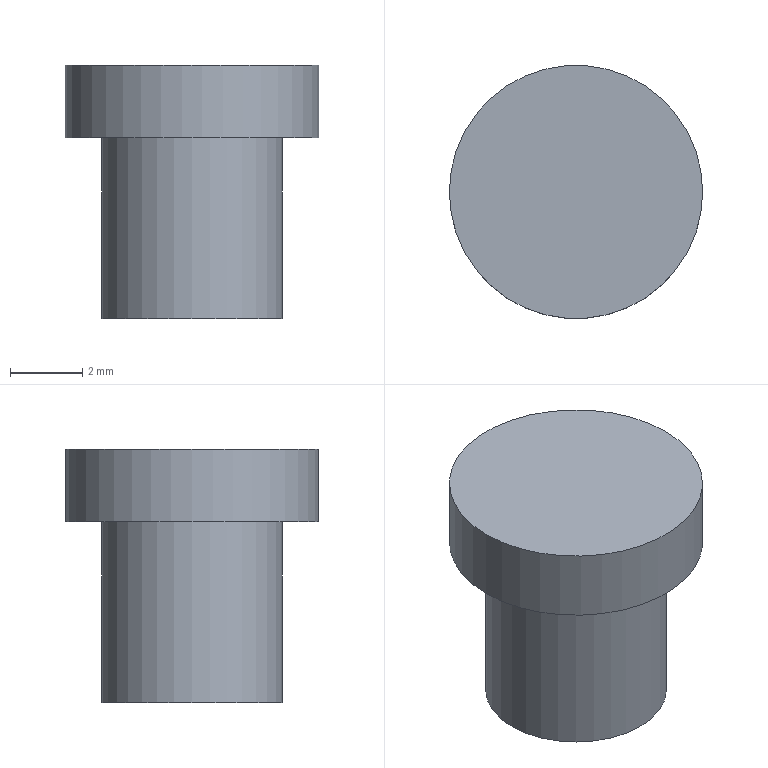Part | NX | features CYLINDER 2, DATUM_CSYS 1 | 1 solid | 5 faces | box 7 x 7 x 7 mm | volume 175.144 mm3 | plane 3 | cylinder 2 | commonest cylinder face diameters 5 x1 7 x1
STEP:
#1=CARTESIAN_POINT('',(2.5,0.,0.));
#2=VERTEX_POINT('',#1);
#3=CARTESIAN_POINT('',(0.,0.,0.));
#4=DIRECTION('',(0.,0.,1.));
#5=DIRECTION('',(1.,0.,0.));
#6=AXIS2_PLACEMENT_3D('',#3,#4,#5);
#7=CIRCLE('',#6,2.5);
#8=EDGE_CURVE('',#2,#2,#7,.T.);
#9=ORIENTED_EDGE('',*,*,#8,.F.);
#10=EDGE_LOOP('',(#9));
#11=FACE_BOUND('',#10,.T.);
#12=CARTESIAN_POINT('',(0.,0.,0.));
#13=DIRECTION('',(0.,0.,-1.));
#14=DIRECTION('',(-1.,0.,0.));
#15=AXIS2_PLACEMENT_3D('',#12,#13,#14);
#16=PLANE('',#15);
#17=ADVANCED_FACE('',(#11),#16,.T.);
#18=CARTESIAN_POINT('',(2.5,0.,5.));
#19=VERTEX_POINT('',#18);
#20=CARTESIAN_POINT('',(0.,0.,5.));
#21=DIRECTION('',(0.,0.,-1.));
#22=DIRECTION('',(1.,0.,0.));
#23=AXIS2_PLACEMENT_3D('',#20,#21,#22);
#24=CIRCLE('',#23,2.5);
#25=EDGE_CURVE('',#19,#19,#24,.T.);
#26=ORIENTED_EDGE('',*,*,#25,.T.);
#27=EDGE_LOOP('',(#26));
#28=FACE_BOUND('',#27,.T.);
#29=ORIENTED_EDGE('',*,*,#8,.T.);
#30=EDGE_LOOP('',(#29));
#31=FACE_BOUND('',#30,.T.);
#32=CARTESIAN_POINT('',(0.,0.,0.));
#33=DIRECTION('',(0.,0.,1.));
#34=DIRECTION('',(1.,0.,0.));
#35=AXIS2_PLACEMENT_3D('',#32,#33,#34);
#36=CYLINDRICAL_SURFACE('',#35,2.5);
#37=ADVANCED_FACE('',(#28,#31),#36,.T.);
#38=CARTESIAN_POINT('',(3.5,0.,7.));
#39=VERTEX_POINT('',#38);
#40=CARTESIAN_POINT('',(0.,0.,7.));
#41=DIRECTION('',(0.,0.,-1.));
#42=DIRECTION('',(1.,0.,0.));
#43=AXIS2_PLACEMENT_3D('',#40,#41,#42);
#44=CIRCLE('',#43,3.5);
#45=EDGE_CURVE('',#39,#39,#44,.T.);
#46=ORIENTED_EDGE('',*,*,#45,.F.);
#47=EDGE_LOOP('',(#46));
#48=FACE_BOUND('',#47,.T.);
#49=CARTESIAN_POINT('',(0.,0.,7.));
#50=DIRECTION('',(0.,0.,1.));
#51=DIRECTION('',(1.,0.,0.));
#52=AXIS2_PLACEMENT_3D('',#49,#50,#51);
#53=PLANE('',#52);
#54=ADVANCED_FACE('',(#48),#53,.T.);
#55=ORIENTED_EDGE('',*,*,#25,.F.);
#56=EDGE_LOOP('',(#55));
#57=FACE_BOUND('',#56,.T.);
#58=CARTESIAN_POINT('',(3.5,0.,5.));
#59=VERTEX_POINT('',#58);
#60=CARTESIAN_POINT('',(0.,0.,5.));
#61=DIRECTION('',(0.,0.,1.));
#62=DIRECTION('',(1.,0.,0.));
#63=AXIS2_PLACEMENT_3D('',#60,#61,#62);
#64=CIRCLE('',#63,3.5);
#65=EDGE_CURVE('',#59,#59,#64,.T.);
#66=ORIENTED_EDGE('',*,*,#65,.F.);
#67=EDGE_LOOP('',(#66));
#68=FACE_BOUND('',#67,.T.);
#69=CARTESIAN_POINT('',(0.,0.,5.));
#70=DIRECTION('',(0.,0.,-1.));
#71=DIRECTION('',(-1.,0.,0.));
#72=AXIS2_PLACEMENT_3D('',#69,#70,#71);
#73=PLANE('',#72);
#74=ADVANCED_FACE('',(#57,#68),#73,.T.);
#75=ORIENTED_EDGE('',*,*,#45,.T.);
#76=EDGE_LOOP('',(#75));
#77=FACE_BOUND('',#76,.T.);
#78=ORIENTED_EDGE('',*,*,#65,.T.);
#79=EDGE_LOOP('',(#78));
#80=FACE_BOUND('',#79,.T.);
#81=CARTESIAN_POINT('',(0.,0.,5.));
#82=DIRECTION('',(0.,0.,1.));
#83=DIRECTION('',(1.,0.,0.));
#84=AXIS2_PLACEMENT_3D('',#81,#82,#83);
#85=CYLINDRICAL_SURFACE('',#84,3.5);
#86=ADVANCED_FACE('',(#77,#80),#85,.T.);
#87=CLOSED_SHELL('',(#17,#37,#54,#74,#86));
#88=MANIFOLD_SOLID_BREP('',#87);
#89=(LENGTH_UNIT()NAMED_UNIT(*)SI_UNIT(.MILLI.,.METRE.));
#90=UNCERTAINTY_MEASURE_WITH_UNIT(LENGTH_MEASURE(0.00001),#89,'','');
#91=(NAMED_UNIT(*)PLANE_ANGLE_UNIT()SI_UNIT($,.RADIAN.));
#92=(NAMED_UNIT(*)SI_UNIT($,.STERADIAN.)SOLID_ANGLE_UNIT());
#93=(GEOMETRIC_REPRESENTATION_CONTEXT(3)GLOBAL_UNCERTAINTY_ASSIGNED_CONTEXT((#90))GLOBAL_UNIT_ASSIGNED_CONTEXT((#89,#91,#92))REPRESENTATION_CONTEXT('',''));
#94=ADVANCED_BREP_SHAPE_REPRESENTATION('',(#88),#93);